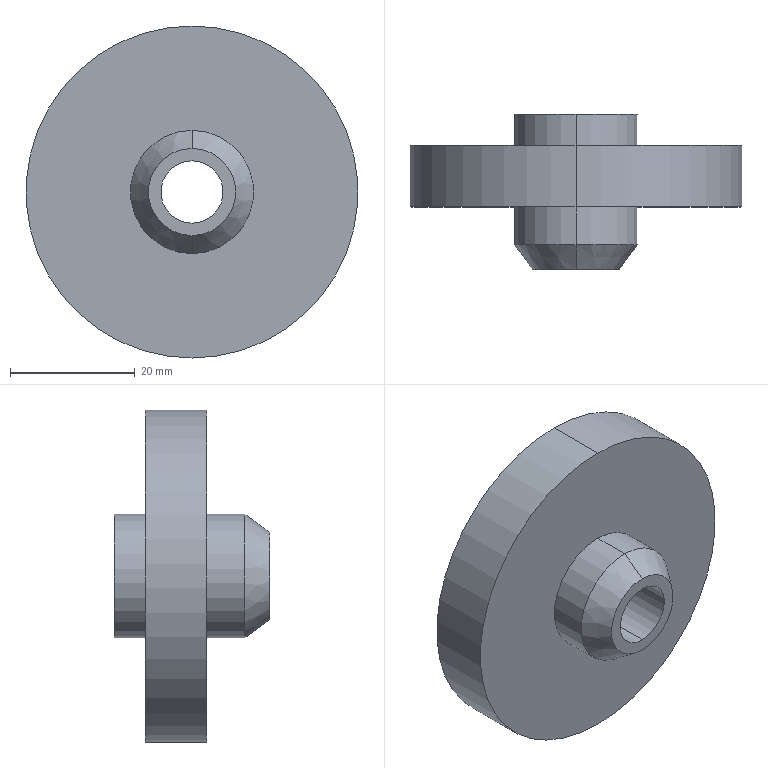Part | STEP file | Guide wheel mechanism revised.sldasm-Part-69 | 1 solid | 16 faces | box 53.3 x 25 x 53.3 mm | volume 24281 mm3 | cylinder 8 | cone 4 | plane 4 | commonest cylinder face diameters 19.8 x4 10 x2 53.3 x2
STEP:
#1=CARTESIAN_POINT('',(0.,15.,5.));
#2=VERTEX_POINT('',#1);
#3=CARTESIAN_POINT('',(0.,15.,-5.));
#4=VERTEX_POINT('',#3);
#5=CARTESIAN_POINT('',(0.,15.,0.));
#6=DIRECTION('',(0.,-1.,0.));
#7=DIRECTION('',(0.,0.,-1.));
#8=AXIS2_PLACEMENT_3D('',#5,#6,#7);
#9=CIRCLE('',#8,5.);
#10=EDGE_CURVE('',#2,#4,#9,.T.);
#11=ORIENTED_EDGE('',*,*,#10,.F.);
#12=CARTESIAN_POINT('',(0.,-5.,5.));
#13=VERTEX_POINT('',#12);
#14=CARTESIAN_POINT('',(0.,0.,5.));
#15=DIRECTION('',(0.,-1.,0.));
#16=VECTOR('',#15,1000.);
#17=LINE('',#14,#16);
#18=EDGE_CURVE('',#2,#13,#17,.T.);
#19=ORIENTED_EDGE('',*,*,#18,.T.);
#20=CARTESIAN_POINT('',(0.,-5.,-5.));
#21=VERTEX_POINT('',#20);
#22=CARTESIAN_POINT('',(0.,-5.,0.));
#23=DIRECTION('',(0.,-1.,0.));
#24=DIRECTION('',(0.,0.,-1.));
#25=AXIS2_PLACEMENT_3D('',#22,#23,#24);
#26=CIRCLE('',#25,5.);
#27=EDGE_CURVE('',#13,#21,#26,.T.);
#28=ORIENTED_EDGE('',*,*,#27,.T.);
#29=CARTESIAN_POINT('',(0.,0.,-5.));
#30=DIRECTION('',(0.,-1.,0.));
#31=VECTOR('',#30,1000.);
#32=LINE('',#29,#31);
#33=EDGE_CURVE('',#4,#21,#32,.T.);
#34=ORIENTED_EDGE('',*,*,#33,.F.);
#35=EDGE_LOOP('',(#11,#19,#28,#34));
#36=FACE_OUTER_BOUND('',#35,.T.);
#37=CARTESIAN_POINT('',(0.,0.,0.));
#38=DIRECTION('',(0.,-1.,0.));
#39=DIRECTION('',(0.,0.,-1.));
#40=AXIS2_PLACEMENT_3D('',#37,#38,#39);
#41=CYLINDRICAL_SURFACE('',#40,5.);
#42=ADVANCED_FACE('',(#36),#41,.F.);
#43=ORIENTED_EDGE('',*,*,#10,.T.);
#44=CARTESIAN_POINT('',(0.,20.,-6.9));
#45=VERTEX_POINT('',#44);
#46=CARTESIAN_POINT('',(0.,15.,-5.));
#47=DIRECTION('',(0.,0.9348,-0.3552));
#48=VECTOR('',#47,1000.);
#49=LINE('',#46,#48);
#50=EDGE_CURVE('',#4,#45,#49,.T.);
#51=ORIENTED_EDGE('',*,*,#50,.T.);
#52=CARTESIAN_POINT('',(0.,20.,6.9));
#53=VERTEX_POINT('',#52);
#54=CARTESIAN_POINT('',(0.,20.,0.));
#55=DIRECTION('',(0.,-1.,0.));
#56=DIRECTION('',(0.,0.,-1.));
#57=AXIS2_PLACEMENT_3D('',#54,#55,#56);
#58=CIRCLE('',#57,6.9);
#59=EDGE_CURVE('',#53,#45,#58,.T.);
#60=ORIENTED_EDGE('',*,*,#59,.F.);
#61=CARTESIAN_POINT('',(0.,15.,5.));
#62=DIRECTION('',(0.,0.9348,0.3552));
#63=VECTOR('',#62,1000.);
#64=LINE('',#61,#63);
#65=EDGE_CURVE('',#2,#53,#64,.T.);
#66=ORIENTED_EDGE('',*,*,#65,.F.);
#67=EDGE_LOOP('',(#43,#51,#60,#66));
#68=FACE_OUTER_BOUND('',#67,.T.);
#69=CARTESIAN_POINT('',(0.,15.,0.));
#70=DIRECTION('',(0.,1.,0.));
#71=DIRECTION('',(0.,0.,1.));
#72=AXIS2_PLACEMENT_3D('',#69,#70,#71);
#73=CONICAL_SURFACE('',#72,5.,0.3631);
#74=ADVANCED_FACE('',(#68),#73,.F.);
#75=CARTESIAN_POINT('',(0.,20.,-9.9));
#76=VERTEX_POINT('',#75);
#77=CARTESIAN_POINT('',(0.,20.,9.9));
#78=VERTEX_POINT('',#77);
#79=CARTESIAN_POINT('',(0.,20.,0.));
#80=DIRECTION('',(0.,-1.,0.));
#81=DIRECTION('',(0.,0.,-1.));
#82=AXIS2_PLACEMENT_3D('',#79,#80,#81);
#83=CIRCLE('',#82,9.9);
#84=EDGE_CURVE('',#76,#78,#83,.T.);
#85=ORIENTED_EDGE('',*,*,#84,.T.);
#86=CARTESIAN_POINT('',(0.,15.,9.9));
#87=VERTEX_POINT('',#86);
#88=CARTESIAN_POINT('',(0.,0.,9.9));
#89=DIRECTION('',(0.,-1.,0.));
#90=VECTOR('',#89,1000.);
#91=LINE('',#88,#90);
#92=EDGE_CURVE('',#78,#87,#91,.T.);
#93=ORIENTED_EDGE('',*,*,#92,.T.);
#94=CARTESIAN_POINT('',(0.,15.,-9.9));
#95=VERTEX_POINT('',#94);
#96=CARTESIAN_POINT('',(0.,15.,0.));
#97=DIRECTION('',(0.,-1.,0.));
#98=DIRECTION('',(0.,0.,-1.));
#99=AXIS2_PLACEMENT_3D('',#96,#97,#98);
#100=CIRCLE('',#99,9.9);
#101=EDGE_CURVE('',#95,#87,#100,.T.);
#102=ORIENTED_EDGE('',*,*,#101,.F.);
#103=CARTESIAN_POINT('',(0.,0.,-9.9));
#104=DIRECTION('',(0.,-1.,0.));
#105=VECTOR('',#104,1000.);
#106=LINE('',#103,#105);
#107=EDGE_CURVE('',#76,#95,#106,.T.);
#108=ORIENTED_EDGE('',*,*,#107,.F.);
#109=EDGE_LOOP('',(#85,#93,#102,#108));
#110=FACE_OUTER_BOUND('',#109,.T.);
#111=CARTESIAN_POINT('',(0.,0.,0.));
#112=DIRECTION('',(0.,-1.,0.));
#113=DIRECTION('',(0.,0.,-1.));
#114=AXIS2_PLACEMENT_3D('',#111,#112,#113);
#115=CYLINDRICAL_SURFACE('',#114,9.9);
#116=ADVANCED_FACE('',(#110),#115,.T.);
#117=CARTESIAN_POINT('',(0.,15.,-26.65));
#118=VERTEX_POINT('',#117);
#119=CARTESIAN_POINT('',(0.,15.,26.65));
#120=VERTEX_POINT('',#119);
#121=CARTESIAN_POINT('',(0.,15.,0.));
#122=DIRECTION('',(0.,-1.,0.));
#123=DIRECTION('',(0.,0.,-1.));
#124=AXIS2_PLACEMENT_3D('',#121,#122,#123);
#125=CIRCLE('',#124,26.65);
#126=EDGE_CURVE('',#118,#120,#125,.T.);
#127=ORIENTED_EDGE('',*,*,#126,.T.);
#128=CARTESIAN_POINT('',(0.,5.1,26.65));
#129=VERTEX_POINT('',#128);
#130=CARTESIAN_POINT('',(0.,0.,26.65));
#131=DIRECTION('',(0.,-1.,0.));
#132=VECTOR('',#131,1000.);
#133=LINE('',#130,#132);
#134=EDGE_CURVE('',#120,#129,#133,.T.);
#135=ORIENTED_EDGE('',*,*,#134,.T.);
#136=CARTESIAN_POINT('',(0.,5.1,-26.65));
#137=VERTEX_POINT('',#136);
#138=CARTESIAN_POINT('',(0.,5.1,0.));
#139=DIRECTION('',(0.,-1.,0.));
#140=DIRECTION('',(0.,0.,-1.));
#141=AXIS2_PLACEMENT_3D('',#138,#139,#140);
#142=CIRCLE('',#141,26.65);
#143=EDGE_CURVE('',#137,#129,#142,.T.);
#144=ORIENTED_EDGE('',*,*,#143,.F.);
#145=CARTESIAN_POINT('',(0.,0.,-26.65));
#146=DIRECTION('',(0.,-1.,0.));
#147=VECTOR('',#146,1000.);
#148=LINE('',#145,#147);
#149=EDGE_CURVE('',#118,#137,#148,.T.);
#150=ORIENTED_EDGE('',*,*,#149,.F.);
#151=EDGE_LOOP('',(#127,#135,#144,#150));
#152=FACE_OUTER_BOUND('',#151,.T.);
#153=CARTESIAN_POINT('',(0.,0.,0.));
#154=DIRECTION('',(0.,-1.,0.));
#155=DIRECTION('',(0.,0.,-1.));
#156=AXIS2_PLACEMENT_3D('',#153,#154,#155);
#157=CYLINDRICAL_SURFACE('',#156,26.65);
#158=ADVANCED_FACE('',(#152),#157,.T.);
#159=CARTESIAN_POINT('',(0.,5.1,-9.9));
#160=VERTEX_POINT('',#159);
#161=CARTESIAN_POINT('',(0.,5.1,9.9));
#162=VERTEX_POINT('',#161);
#163=CARTESIAN_POINT('',(0.,5.1,0.));
#164=DIRECTION('',(0.,-1.,0.));
#165=DIRECTION('',(0.,0.,-1.));
#166=AXIS2_PLACEMENT_3D('',#163,#164,#165);
#167=CIRCLE('',#166,9.9);
#168=EDGE_CURVE('',#160,#162,#167,.T.);
#169=ORIENTED_EDGE('',*,*,#168,.T.);
#170=CARTESIAN_POINT('',(0.,-1.,9.9));
#171=VERTEX_POINT('',#170);
#172=CARTESIAN_POINT('',(0.,0.,9.9));
#173=DIRECTION('',(0.,-1.,0.));
#174=VECTOR('',#173,1000.);
#175=LINE('',#172,#174);
#176=EDGE_CURVE('',#162,#171,#175,.T.);
#177=ORIENTED_EDGE('',*,*,#176,.T.);
#178=CARTESIAN_POINT('',(0.,-1.,-9.9));
#179=VERTEX_POINT('',#178);
#180=CARTESIAN_POINT('',(0.,-1.,0.));
#181=DIRECTION('',(0.,-1.,0.));
#182=DIRECTION('',(0.,0.,-1.));
#183=AXIS2_PLACEMENT_3D('',#180,#181,#182);
#184=CIRCLE('',#183,9.9);
#185=EDGE_CURVE('',#179,#171,#184,.T.);
#186=ORIENTED_EDGE('',*,*,#185,.F.);
#187=CARTESIAN_POINT('',(0.,0.,-9.9));
#188=DIRECTION('',(0.,-1.,0.));
#189=VECTOR('',#188,1000.);
#190=LINE('',#187,#189);
#191=EDGE_CURVE('',#160,#179,#190,.T.);
#192=ORIENTED_EDGE('',*,*,#191,.F.);
#193=EDGE_LOOP('',(#169,#177,#186,#192));
#194=FACE_OUTER_BOUND('',#193,.T.);
#195=CARTESIAN_POINT('',(0.,0.,0.));
#196=DIRECTION('',(0.,-1.,0.));
#197=DIRECTION('',(0.,0.,-1.));
#198=AXIS2_PLACEMENT_3D('',#195,#196,#197);
#199=CYLINDRICAL_SURFACE('',#198,9.9);
#200=ADVANCED_FACE('',(#194),#199,.T.);
#201=CARTESIAN_POINT('',(0.,-5.,-7.));
#202=VERTEX_POINT('',#201);
#203=CARTESIAN_POINT('',(0.,-5.,7.));
#204=VERTEX_POINT('',#203);
#205=CARTESIAN_POINT('',(0.,-5.,0.));
#206=DIRECTION('',(0.,-1.,0.));
#207=DIRECTION('',(0.,0.,-1.));
#208=AXIS2_PLACEMENT_3D('',#205,#206,#207);
#209=CIRCLE('',#208,7.);
#210=EDGE_CURVE('',#202,#204,#209,.T.);
#211=ORIENTED_EDGE('',*,*,#210,.F.);
#212=CARTESIAN_POINT('',(0.,-1.,-9.9));
#213=DIRECTION('',(0.,0.8096,-0.587));
#214=VECTOR('',#213,1000.);
#215=LINE('',#212,#214);
#216=EDGE_CURVE('',#202,#179,#215,.T.);
#217=ORIENTED_EDGE('',*,*,#216,.T.);
#218=ORIENTED_EDGE('',*,*,#185,.T.);
#219=CARTESIAN_POINT('',(0.,-1.,9.9));
#220=DIRECTION('',(0.,0.8096,0.587));
#221=VECTOR('',#220,1000.);
#222=LINE('',#219,#221);
#223=EDGE_CURVE('',#204,#171,#222,.T.);
#224=ORIENTED_EDGE('',*,*,#223,.F.);
#225=EDGE_LOOP('',(#211,#217,#218,#224));
#226=FACE_OUTER_BOUND('',#225,.T.);
#227=CARTESIAN_POINT('',(0.,-1.,0.));
#228=DIRECTION('',(0.,1.,0.));
#229=DIRECTION('',(0.,0.,1.));
#230=AXIS2_PLACEMENT_3D('',#227,#228,#229);
#231=CONICAL_SURFACE('',#230,9.9,0.6273);
#232=ADVANCED_FACE('',(#226),#231,.T.);
#233=CARTESIAN_POINT('',(0.,-5.,0.));
#234=DIRECTION('',(0.,-1.,0.));
#235=DIRECTION('',(0.,0.,-1.));
#236=AXIS2_PLACEMENT_3D('',#233,#234,#235);
#237=CIRCLE('',#236,5.);
#238=EDGE_CURVE('',#21,#13,#237,.T.);
#239=ORIENTED_EDGE('',*,*,#238,.F.);
#240=ORIENTED_EDGE('',*,*,#27,.F.);
#241=EDGE_LOOP('',(#239,#240));
#242=FACE_BOUND('',#241,.T.);
#243=CARTESIAN_POINT('',(0.,-5.,0.));
#244=DIRECTION('',(0.,-1.,0.));
#245=DIRECTION('',(0.,0.,-1.));
#246=AXIS2_PLACEMENT_3D('',#243,#244,#245);
#247=CIRCLE('',#246,7.);
#248=EDGE_CURVE('',#204,#202,#247,.T.);
#249=ORIENTED_EDGE('',*,*,#248,.T.);
#250=ORIENTED_EDGE('',*,*,#210,.T.);
#251=EDGE_LOOP('',(#249,#250));
#252=FACE_OUTER_BOUND('',#251,.T.);
#253=CARTESIAN_POINT('',(0.,-5.,0.));
#254=DIRECTION('',(0.,1.,0.));
#255=DIRECTION('',(0.,0.,1.));
#256=AXIS2_PLACEMENT_3D('',#253,#254,#255);
#257=PLANE('',#256);
#258=ADVANCED_FACE('',(#242,#252),#257,.F.);
#259=ORIENTED_EDGE('',*,*,#216,.F.);
#260=ORIENTED_EDGE('',*,*,#248,.F.);
#261=ORIENTED_EDGE('',*,*,#223,.T.);
#262=CARTESIAN_POINT('',(0.,-1.,0.));
#263=DIRECTION('',(0.,-1.,0.));
#264=DIRECTION('',(0.,0.,-1.));
#265=AXIS2_PLACEMENT_3D('',#262,#263,#264);
#266=CIRCLE('',#265,9.9);
#267=EDGE_CURVE('',#171,#179,#266,.T.);
#268=ORIENTED_EDGE('',*,*,#267,.T.);
#269=EDGE_LOOP('',(#259,#260,#261,#268));
#270=FACE_OUTER_BOUND('',#269,.T.);
#271=CARTESIAN_POINT('',(0.,-1.,0.));
#272=DIRECTION('',(0.,1.,0.));
#273=DIRECTION('',(0.,0.,1.));
#274=AXIS2_PLACEMENT_3D('',#271,#272,#273);
#275=CONICAL_SURFACE('',#274,9.9,0.6273);
#276=ADVANCED_FACE('',(#270),#275,.T.);
#277=ORIENTED_EDGE('',*,*,#176,.F.);
#278=CARTESIAN_POINT('',(0.,5.1,0.));
#279=DIRECTION('',(0.,-1.,0.));
#280=DIRECTION('',(0.,0.,-1.));
#281=AXIS2_PLACEMENT_3D('',#278,#279,#280);
#282=CIRCLE('',#281,9.9);
#283=EDGE_CURVE('',#162,#160,#282,.T.);
#284=ORIENTED_EDGE('',*,*,#283,.T.);
#285=ORIENTED_EDGE('',*,*,#191,.T.);
#286=ORIENTED_EDGE('',*,*,#267,.F.);
#287=EDGE_LOOP('',(#277,#284,#285,#286));
#288=FACE_OUTER_BOUND('',#287,.T.);
#289=CARTESIAN_POINT('',(0.,0.,0.));
#290=DIRECTION('',(0.,-1.,0.));
#291=DIRECTION('',(0.,0.,-1.));
#292=AXIS2_PLACEMENT_3D('',#289,#290,#291);
#293=CYLINDRICAL_SURFACE('',#292,9.9);
#294=ADVANCED_FACE('',(#288),#293,.T.);
#295=ORIENTED_EDGE('',*,*,#143,.T.);
#296=CARTESIAN_POINT('',(0.,5.1,0.));
#297=DIRECTION('',(0.,-1.,0.));
#298=DIRECTION('',(0.,0.,-1.));
#299=AXIS2_PLACEMENT_3D('',#296,#297,#298);
#300=CIRCLE('',#299,26.65);
#301=EDGE_CURVE('',#129,#137,#300,.T.);
#302=ORIENTED_EDGE('',*,*,#301,.T.);
#303=EDGE_LOOP('',(#295,#302));
#304=FACE_OUTER_BOUND('',#303,.T.);
#305=ORIENTED_EDGE('',*,*,#168,.F.);
#306=ORIENTED_EDGE('',*,*,#283,.F.);
#307=EDGE_LOOP('',(#305,#306));
#308=FACE_BOUND('',#307,.T.);
#309=CARTESIAN_POINT('',(0.,5.1,0.));
#310=DIRECTION('',(0.,-1.,0.));
#311=DIRECTION('',(0.,0.,-1.));
#312=AXIS2_PLACEMENT_3D('',#309,#310,#311);
#313=PLANE('',#312);
#314=ADVANCED_FACE('',(#304,#308),#313,.T.);
#315=ORIENTED_EDGE('',*,*,#134,.F.);
#316=CARTESIAN_POINT('',(0.,15.,0.));
#317=DIRECTION('',(0.,-1.,0.));
#318=DIRECTION('',(0.,0.,-1.));
#319=AXIS2_PLACEMENT_3D('',#316,#317,#318);
#320=CIRCLE('',#319,26.65);
#321=EDGE_CURVE('',#120,#118,#320,.T.);
#322=ORIENTED_EDGE('',*,*,#321,.T.);
#323=ORIENTED_EDGE('',*,*,#149,.T.);
#324=ORIENTED_EDGE('',*,*,#301,.F.);
#325=EDGE_LOOP('',(#315,#322,#323,#324));
#326=FACE_OUTER_BOUND('',#325,.T.);
#327=CARTESIAN_POINT('',(0.,0.,0.));
#328=DIRECTION('',(0.,-1.,0.));
#329=DIRECTION('',(0.,0.,-1.));
#330=AXIS2_PLACEMENT_3D('',#327,#328,#329);
#331=CYLINDRICAL_SURFACE('',#330,26.65);
#332=ADVANCED_FACE('',(#326),#331,.T.);
#333=ORIENTED_EDGE('',*,*,#101,.T.);
#334=CARTESIAN_POINT('',(0.,15.,0.));
#335=DIRECTION('',(0.,-1.,0.));
#336=DIRECTION('',(0.,0.,-1.));
#337=AXIS2_PLACEMENT_3D('',#334,#335,#336);
#338=CIRCLE('',#337,9.9);
#339=EDGE_CURVE('',#87,#95,#338,.T.);
#340=ORIENTED_EDGE('',*,*,#339,.T.);
#341=EDGE_LOOP('',(#333,#340));
#342=FACE_BOUND('',#341,.T.);
#343=ORIENTED_EDGE('',*,*,#126,.F.);
#344=ORIENTED_EDGE('',*,*,#321,.F.);
#345=EDGE_LOOP('',(#343,#344));
#346=FACE_OUTER_BOUND('',#345,.T.);
#347=CARTESIAN_POINT('',(0.,15.,0.));
#348=DIRECTION('',(0.,1.,0.));
#349=DIRECTION('',(0.,0.,1.));
#350=AXIS2_PLACEMENT_3D('',#347,#348,#349);
#351=PLANE('',#350);
#352=ADVANCED_FACE('',(#342,#346),#351,.T.);
#353=ORIENTED_EDGE('',*,*,#92,.F.);
#354=CARTESIAN_POINT('',(0.,20.,0.));
#355=DIRECTION('',(0.,-1.,0.));
#356=DIRECTION('',(0.,0.,-1.));
#357=AXIS2_PLACEMENT_3D('',#354,#355,#356);
#358=CIRCLE('',#357,9.9);
#359=EDGE_CURVE('',#78,#76,#358,.T.);
#360=ORIENTED_EDGE('',*,*,#359,.T.);
#361=ORIENTED_EDGE('',*,*,#107,.T.);
#362=ORIENTED_EDGE('',*,*,#339,.F.);
#363=EDGE_LOOP('',(#353,#360,#361,#362));
#364=FACE_OUTER_BOUND('',#363,.T.);
#365=CARTESIAN_POINT('',(0.,0.,0.));
#366=DIRECTION('',(0.,-1.,0.));
#367=DIRECTION('',(0.,0.,-1.));
#368=AXIS2_PLACEMENT_3D('',#365,#366,#367);
#369=CYLINDRICAL_SURFACE('',#368,9.9);
#370=ADVANCED_FACE('',(#364),#369,.T.);
#371=ORIENTED_EDGE('',*,*,#59,.T.);
#372=CARTESIAN_POINT('',(0.,20.,0.));
#373=DIRECTION('',(0.,-1.,0.));
#374=DIRECTION('',(0.,0.,-1.));
#375=AXIS2_PLACEMENT_3D('',#372,#373,#374);
#376=CIRCLE('',#375,6.9);
#377=EDGE_CURVE('',#45,#53,#376,.T.);
#378=ORIENTED_EDGE('',*,*,#377,.T.);
#379=EDGE_LOOP('',(#371,#378));
#380=FACE_BOUND('',#379,.T.);
#381=ORIENTED_EDGE('',*,*,#84,.F.);
#382=ORIENTED_EDGE('',*,*,#359,.F.);
#383=EDGE_LOOP('',(#381,#382));
#384=FACE_OUTER_BOUND('',#383,.T.);
#385=CARTESIAN_POINT('',(0.,20.,0.));
#386=DIRECTION('',(0.,1.,0.));
#387=DIRECTION('',(0.,0.,1.));
#388=AXIS2_PLACEMENT_3D('',#385,#386,#387);
#389=PLANE('',#388);
#390=ADVANCED_FACE('',(#380,#384),#389,.T.);
#391=ORIENTED_EDGE('',*,*,#50,.F.);
#392=CARTESIAN_POINT('',(0.,15.,0.));
#393=DIRECTION('',(0.,-1.,0.));
#394=DIRECTION('',(0.,0.,-1.));
#395=AXIS2_PLACEMENT_3D('',#392,#393,#394);
#396=CIRCLE('',#395,5.);
#397=EDGE_CURVE('',#4,#2,#396,.T.);
#398=ORIENTED_EDGE('',*,*,#397,.T.);
#399=ORIENTED_EDGE('',*,*,#65,.T.);
#400=ORIENTED_EDGE('',*,*,#377,.F.);
#401=EDGE_LOOP('',(#391,#398,#399,#400));
#402=FACE_OUTER_BOUND('',#401,.T.);
#403=CARTESIAN_POINT('',(0.,15.,0.));
#404=DIRECTION('',(0.,1.,0.));
#405=DIRECTION('',(0.,0.,1.));
#406=AXIS2_PLACEMENT_3D('',#403,#404,#405);
#407=CONICAL_SURFACE('',#406,5.,0.3631);
#408=ADVANCED_FACE('',(#402),#407,.F.);
#409=ORIENTED_EDGE('',*,*,#18,.F.);
#410=ORIENTED_EDGE('',*,*,#397,.F.);
#411=ORIENTED_EDGE('',*,*,#33,.T.);
#412=ORIENTED_EDGE('',*,*,#238,.T.);
#413=EDGE_LOOP('',(#409,#410,#411,#412));
#414=FACE_OUTER_BOUND('',#413,.T.);
#415=CARTESIAN_POINT('',(0.,0.,0.));
#416=DIRECTION('',(0.,-1.,0.));
#417=DIRECTION('',(0.,0.,-1.));
#418=AXIS2_PLACEMENT_3D('',#415,#416,#417);
#419=CYLINDRICAL_SURFACE('',#418,5.);
#420=ADVANCED_FACE('',(#414),#419,.F.);
#421=CLOSED_SHELL('',(#42,#74,#116,#158,#200,#232,#258,#276,#294,#314,#332,#352,#370,#390,#408,#420));
#422=MANIFOLD_SOLID_BREP('',#421);
#423=CARTESIAN_POINT('',(0.,0.,0.));
#424=DIRECTION('',(0.,0.,1.));
#425=DIRECTION('',(1.,0.,0.));
#426=AXIS2_PLACEMENT_3D('',#423,#424,#425);
#427=(LENGTH_UNIT()NAMED_UNIT(*)SI_UNIT(.MILLI.,.METRE.));
#428=UNCERTAINTY_MEASURE_WITH_UNIT(LENGTH_MEASURE(0.00001),#427,'','');
#429=(NAMED_UNIT(*)PLANE_ANGLE_UNIT()SI_UNIT($,.RADIAN.));
#430=(NAMED_UNIT(*)SI_UNIT($,.STERADIAN.)SOLID_ANGLE_UNIT());
#431=(GEOMETRIC_REPRESENTATION_CONTEXT(3)GLOBAL_UNCERTAINTY_ASSIGNED_CONTEXT((#428))GLOBAL_UNIT_ASSIGNED_CONTEXT((#427,#429,#430))REPRESENTATION_CONTEXT('',''));
#432=ADVANCED_BREP_SHAPE_REPRESENTATION('',(#422,#426),#431);